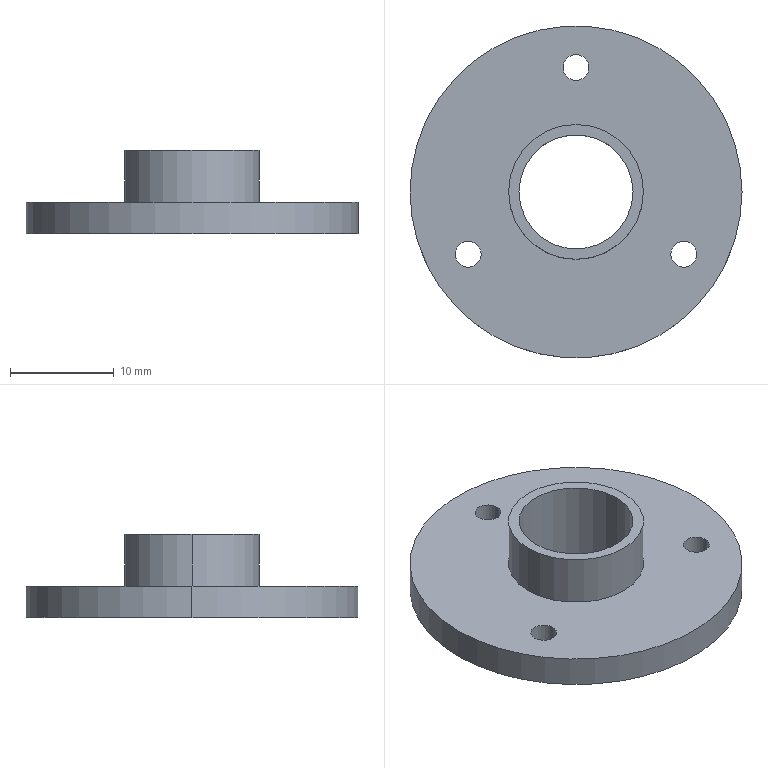Part | SolidWorks | features ICE 3, Extrusion 1, HoleWzd 1 | 1 solid | 15 faces | box 32 x 32 x 8 mm | volume 2272 mm3 | cylinder 12 | plane 3 | commonest cylinder face diameters 2.5 x6 11 x2 13 x2 32 x2
STEP:
#1=CARTESIAN_POINT('',(-1.25,12.,3.));
#2=VERTEX_POINT('',#1);
#3=CARTESIAN_POINT('',(1.25,12.,3.));
#4=VERTEX_POINT('',#3);
#5=CARTESIAN_POINT('',(0.,12.,3.));
#6=DIRECTION('',(0.,0.,1.));
#7=DIRECTION('',(1.,0.,0.));
#8=AXIS2_PLACEMENT_3D('',#5,#6,#7);
#9=CIRCLE('',#8,1.25);
#10=EDGE_CURVE('',#2,#4,#9,.T.);
#11=ORIENTED_EDGE('',*,*,#10,.T.);
#12=CARTESIAN_POINT('',(1.25,12.,0.));
#13=VERTEX_POINT('',#12);
#14=CARTESIAN_POINT('',(1.25,12.,0.));
#15=DIRECTION('',(0.,0.,-1.));
#16=VECTOR('',#15,1000.);
#17=LINE('',#14,#16);
#18=EDGE_CURVE('',#4,#13,#17,.T.);
#19=ORIENTED_EDGE('',*,*,#18,.T.);
#20=CARTESIAN_POINT('',(-1.25,12.,0.));
#21=VERTEX_POINT('',#20);
#22=CARTESIAN_POINT('',(0.,12.,0.));
#23=DIRECTION('',(0.,0.,-1.));
#24=DIRECTION('',(-1.,0.,0.));
#25=AXIS2_PLACEMENT_3D('',#22,#23,#24);
#26=CIRCLE('',#25,1.25);
#27=EDGE_CURVE('',#13,#21,#26,.T.);
#28=ORIENTED_EDGE('',*,*,#27,.T.);
#29=CARTESIAN_POINT('',(-1.25,12.,0.));
#30=DIRECTION('',(0.,0.,-1.));
#31=VECTOR('',#30,1000.);
#32=LINE('',#29,#31);
#33=EDGE_CURVE('',#2,#21,#32,.T.);
#34=ORIENTED_EDGE('',*,*,#33,.F.);
#35=EDGE_LOOP('',(#11,#19,#28,#34));
#36=FACE_OUTER_BOUND('',#35,.T.);
#37=CARTESIAN_POINT('',(0.,12.,0.));
#38=DIRECTION('',(0.,0.,-1.));
#39=DIRECTION('',(-1.,0.,0.));
#40=AXIS2_PLACEMENT_3D('',#37,#38,#39);
#41=CYLINDRICAL_SURFACE('',#40,1.25);
#42=ADVANCED_FACE('',(#36),#41,.F.);
#43=CARTESIAN_POINT('',(-11.642,-6.,3.));
#44=VERTEX_POINT('',#43);
#45=CARTESIAN_POINT('',(-9.142,-6.,3.));
#46=VERTEX_POINT('',#45);
#47=CARTESIAN_POINT('',(-10.392,-6.,3.));
#48=DIRECTION('',(0.,0.,1.));
#49=DIRECTION('',(1.,0.,0.));
#50=AXIS2_PLACEMENT_3D('',#47,#48,#49);
#51=CIRCLE('',#50,1.25);
#52=EDGE_CURVE('',#44,#46,#51,.T.);
#53=ORIENTED_EDGE('',*,*,#52,.T.);
#54=CARTESIAN_POINT('',(-9.142,-6.,0.));
#55=VERTEX_POINT('',#54);
#56=CARTESIAN_POINT('',(-9.142,-6.,0.));
#57=DIRECTION('',(0.,0.,-1.));
#58=VECTOR('',#57,1000.);
#59=LINE('',#56,#58);
#60=EDGE_CURVE('',#46,#55,#59,.T.);
#61=ORIENTED_EDGE('',*,*,#60,.T.);
#62=CARTESIAN_POINT('',(-11.642,-6.,0.));
#63=VERTEX_POINT('',#62);
#64=CARTESIAN_POINT('',(-10.392,-6.,0.));
#65=DIRECTION('',(0.,0.,-1.));
#66=DIRECTION('',(-1.,0.,0.));
#67=AXIS2_PLACEMENT_3D('',#64,#65,#66);
#68=CIRCLE('',#67,1.25);
#69=EDGE_CURVE('',#55,#63,#68,.T.);
#70=ORIENTED_EDGE('',*,*,#69,.T.);
#71=CARTESIAN_POINT('',(-11.642,-6.,0.));
#72=DIRECTION('',(0.,0.,-1.));
#73=VECTOR('',#72,1000.);
#74=LINE('',#71,#73);
#75=EDGE_CURVE('',#44,#63,#74,.T.);
#76=ORIENTED_EDGE('',*,*,#75,.F.);
#77=EDGE_LOOP('',(#53,#61,#70,#76));
#78=FACE_OUTER_BOUND('',#77,.T.);
#79=CARTESIAN_POINT('',(-10.392,-6.,0.));
#80=DIRECTION('',(0.,0.,-1.));
#81=DIRECTION('',(-1.,0.,0.));
#82=AXIS2_PLACEMENT_3D('',#79,#80,#81);
#83=CYLINDRICAL_SURFACE('',#82,1.25);
#84=ADVANCED_FACE('',(#78),#83,.F.);
#85=CARTESIAN_POINT('',(9.142,-6.,3.));
#86=VERTEX_POINT('',#85);
#87=CARTESIAN_POINT('',(11.642,-6.,3.));
#88=VERTEX_POINT('',#87);
#89=CARTESIAN_POINT('',(10.392,-6.,3.));
#90=DIRECTION('',(0.,0.,1.));
#91=DIRECTION('',(1.,0.,0.));
#92=AXIS2_PLACEMENT_3D('',#89,#90,#91);
#93=CIRCLE('',#92,1.25);
#94=EDGE_CURVE('',#86,#88,#93,.T.);
#95=ORIENTED_EDGE('',*,*,#94,.T.);
#96=CARTESIAN_POINT('',(11.642,-6.,0.));
#97=VERTEX_POINT('',#96);
#98=CARTESIAN_POINT('',(11.642,-6.,0.));
#99=DIRECTION('',(0.,0.,-1.));
#100=VECTOR('',#99,1000.);
#101=LINE('',#98,#100);
#102=EDGE_CURVE('',#88,#97,#101,.T.);
#103=ORIENTED_EDGE('',*,*,#102,.T.);
#104=CARTESIAN_POINT('',(9.142,-6.,0.));
#105=VERTEX_POINT('',#104);
#106=CARTESIAN_POINT('',(10.392,-6.,0.));
#107=DIRECTION('',(0.,0.,-1.));
#108=DIRECTION('',(-1.,0.,0.));
#109=AXIS2_PLACEMENT_3D('',#106,#107,#108);
#110=CIRCLE('',#109,1.25);
#111=EDGE_CURVE('',#97,#105,#110,.T.);
#112=ORIENTED_EDGE('',*,*,#111,.T.);
#113=CARTESIAN_POINT('',(9.142,-6.,0.));
#114=DIRECTION('',(0.,0.,-1.));
#115=VECTOR('',#114,1000.);
#116=LINE('',#113,#115);
#117=EDGE_CURVE('',#86,#105,#116,.T.);
#118=ORIENTED_EDGE('',*,*,#117,.F.);
#119=EDGE_LOOP('',(#95,#103,#112,#118));
#120=FACE_OUTER_BOUND('',#119,.T.);
#121=CARTESIAN_POINT('',(10.392,-6.,0.));
#122=DIRECTION('',(0.,0.,-1.));
#123=DIRECTION('',(-1.,0.,0.));
#124=AXIS2_PLACEMENT_3D('',#121,#122,#123);
#125=CYLINDRICAL_SURFACE('',#124,1.25);
#126=ADVANCED_FACE('',(#120),#125,.F.);
#127=CARTESIAN_POINT('',(-5.5,0.,8.));
#128=VERTEX_POINT('',#127);
#129=CARTESIAN_POINT('',(5.5,0.,8.));
#130=VERTEX_POINT('',#129);
#131=CARTESIAN_POINT('',(0.,0.,8.));
#132=DIRECTION('',(0.,0.,1.));
#133=DIRECTION('',(1.,0.,0.));
#134=AXIS2_PLACEMENT_3D('',#131,#132,#133);
#135=CIRCLE('',#134,5.5);
#136=EDGE_CURVE('',#128,#130,#135,.T.);
#137=ORIENTED_EDGE('',*,*,#136,.T.);
#138=CARTESIAN_POINT('',(5.5,0.,0.));
#139=VERTEX_POINT('',#138);
#140=CARTESIAN_POINT('',(5.5,0.,22.));
#141=DIRECTION('',(0.,0.,-1.));
#142=VECTOR('',#141,1000.);
#143=LINE('',#140,#142);
#144=EDGE_CURVE('',#130,#139,#143,.T.);
#145=ORIENTED_EDGE('',*,*,#144,.T.);
#146=CARTESIAN_POINT('',(-5.5,0.,0.));
#147=VERTEX_POINT('',#146);
#148=CARTESIAN_POINT('',(0.,0.,0.));
#149=DIRECTION('',(0.,0.,-1.));
#150=DIRECTION('',(-1.,0.,0.));
#151=AXIS2_PLACEMENT_3D('',#148,#149,#150);
#152=CIRCLE('',#151,5.5);
#153=EDGE_CURVE('',#139,#147,#152,.T.);
#154=ORIENTED_EDGE('',*,*,#153,.T.);
#155=CARTESIAN_POINT('',(-5.5,0.,22.));
#156=DIRECTION('',(0.,0.,-1.));
#157=VECTOR('',#156,1000.);
#158=LINE('',#155,#157);
#159=EDGE_CURVE('',#128,#147,#158,.T.);
#160=ORIENTED_EDGE('',*,*,#159,.F.);
#161=EDGE_LOOP('',(#137,#145,#154,#160));
#162=FACE_OUTER_BOUND('',#161,.T.);
#163=CARTESIAN_POINT('',(0.,0.,22.));
#164=DIRECTION('',(0.,0.,-1.));
#165=DIRECTION('',(-1.,0.,0.));
#166=AXIS2_PLACEMENT_3D('',#163,#164,#165);
#167=CYLINDRICAL_SURFACE('',#166,5.5);
#168=ADVANCED_FACE('',(#162),#167,.F.);
#169=CARTESIAN_POINT('',(6.5,0.,8.));
#170=VERTEX_POINT('',#169);
#171=CARTESIAN_POINT('',(-6.5,0.,8.));
#172=VERTEX_POINT('',#171);
#173=CARTESIAN_POINT('',(0.,0.,8.));
#174=DIRECTION('',(0.,0.,1.));
#175=DIRECTION('',(1.,0.,0.));
#176=AXIS2_PLACEMENT_3D('',#173,#174,#175);
#177=CIRCLE('',#176,6.5);
#178=EDGE_CURVE('',#170,#172,#177,.T.);
#179=ORIENTED_EDGE('',*,*,#178,.F.);
#180=CARTESIAN_POINT('',(6.5,0.,3.));
#181=VERTEX_POINT('',#180);
#182=CARTESIAN_POINT('',(6.5,0.,8.));
#183=DIRECTION('',(0.,0.,-1.));
#184=VECTOR('',#183,1000.);
#185=LINE('',#182,#184);
#186=EDGE_CURVE('',#170,#181,#185,.T.);
#187=ORIENTED_EDGE('',*,*,#186,.T.);
#188=CARTESIAN_POINT('',(-6.5,0.,3.));
#189=VERTEX_POINT('',#188);
#190=CARTESIAN_POINT('',(0.,0.,3.));
#191=DIRECTION('',(0.,0.,1.));
#192=DIRECTION('',(1.,0.,0.));
#193=AXIS2_PLACEMENT_3D('',#190,#191,#192);
#194=CIRCLE('',#193,6.5);
#195=EDGE_CURVE('',#181,#189,#194,.T.);
#196=ORIENTED_EDGE('',*,*,#195,.T.);
#197=CARTESIAN_POINT('',(-6.5,0.,8.));
#198=DIRECTION('',(0.,0.,-1.));
#199=VECTOR('',#198,1000.);
#200=LINE('',#197,#199);
#201=EDGE_CURVE('',#172,#189,#200,.T.);
#202=ORIENTED_EDGE('',*,*,#201,.F.);
#203=EDGE_LOOP('',(#179,#187,#196,#202));
#204=FACE_OUTER_BOUND('',#203,.T.);
#205=CARTESIAN_POINT('',(0.,0.,8.));
#206=DIRECTION('',(0.,0.,-1.));
#207=DIRECTION('',(-1.,0.,0.));
#208=AXIS2_PLACEMENT_3D('',#205,#206,#207);
#209=CYLINDRICAL_SURFACE('',#208,6.5);
#210=ADVANCED_FACE('',(#204),#209,.T.);
#211=CARTESIAN_POINT('',(16.,0.,3.));
#212=VERTEX_POINT('',#211);
#213=CARTESIAN_POINT('',(-16.,0.,3.));
#214=VERTEX_POINT('',#213);
#215=CARTESIAN_POINT('',(0.,0.,3.));
#216=DIRECTION('',(0.,0.,1.));
#217=DIRECTION('',(1.,0.,0.));
#218=AXIS2_PLACEMENT_3D('',#215,#216,#217);
#219=CIRCLE('',#218,16.);
#220=EDGE_CURVE('',#212,#214,#219,.T.);
#221=ORIENTED_EDGE('',*,*,#220,.F.);
#222=CARTESIAN_POINT('',(16.,0.,0.));
#223=VERTEX_POINT('',#222);
#224=CARTESIAN_POINT('',(16.,0.,3.));
#225=DIRECTION('',(0.,0.,-1.));
#226=VECTOR('',#225,1000.);
#227=LINE('',#224,#226);
#228=EDGE_CURVE('',#212,#223,#227,.T.);
#229=ORIENTED_EDGE('',*,*,#228,.T.);
#230=CARTESIAN_POINT('',(-16.,0.,0.));
#231=VERTEX_POINT('',#230);
#232=CARTESIAN_POINT('',(0.,0.,0.));
#233=DIRECTION('',(0.,0.,1.));
#234=DIRECTION('',(1.,0.,0.));
#235=AXIS2_PLACEMENT_3D('',#232,#233,#234);
#236=CIRCLE('',#235,16.);
#237=EDGE_CURVE('',#223,#231,#236,.T.);
#238=ORIENTED_EDGE('',*,*,#237,.T.);
#239=CARTESIAN_POINT('',(-16.,0.,3.));
#240=DIRECTION('',(0.,0.,-1.));
#241=VECTOR('',#240,1000.);
#242=LINE('',#239,#241);
#243=EDGE_CURVE('',#214,#231,#242,.T.);
#244=ORIENTED_EDGE('',*,*,#243,.F.);
#245=EDGE_LOOP('',(#221,#229,#238,#244));
#246=FACE_OUTER_BOUND('',#245,.T.);
#247=CARTESIAN_POINT('',(0.,0.,3.));
#248=DIRECTION('',(0.,0.,-1.));
#249=DIRECTION('',(-1.,0.,0.));
#250=AXIS2_PLACEMENT_3D('',#247,#248,#249);
#251=CYLINDRICAL_SURFACE('',#250,16.);
#252=ADVANCED_FACE('',(#246),#251,.T.);
#253=ORIENTED_EDGE('',*,*,#228,.F.);
#254=CARTESIAN_POINT('',(0.,0.,3.));
#255=DIRECTION('',(0.,0.,1.));
#256=DIRECTION('',(1.,0.,0.));
#257=AXIS2_PLACEMENT_3D('',#254,#255,#256);
#258=CIRCLE('',#257,16.);
#259=EDGE_CURVE('',#214,#212,#258,.T.);
#260=ORIENTED_EDGE('',*,*,#259,.F.);
#261=ORIENTED_EDGE('',*,*,#243,.T.);
#262=CARTESIAN_POINT('',(0.,0.,0.));
#263=DIRECTION('',(0.,0.,1.));
#264=DIRECTION('',(1.,0.,0.));
#265=AXIS2_PLACEMENT_3D('',#262,#263,#264);
#266=CIRCLE('',#265,16.);
#267=EDGE_CURVE('',#231,#223,#266,.T.);
#268=ORIENTED_EDGE('',*,*,#267,.T.);
#269=EDGE_LOOP('',(#253,#260,#261,#268));
#270=FACE_OUTER_BOUND('',#269,.T.);
#271=CARTESIAN_POINT('',(0.,0.,3.));
#272=DIRECTION('',(0.,0.,-1.));
#273=DIRECTION('',(-1.,0.,0.));
#274=AXIS2_PLACEMENT_3D('',#271,#272,#273);
#275=CYLINDRICAL_SURFACE('',#274,16.);
#276=ADVANCED_FACE('',(#270),#275,.T.);
#277=ORIENTED_EDGE('',*,*,#10,.F.);
#278=CARTESIAN_POINT('',(0.,12.,3.));
#279=DIRECTION('',(0.,0.,1.));
#280=DIRECTION('',(1.,0.,0.));
#281=AXIS2_PLACEMENT_3D('',#278,#279,#280);
#282=CIRCLE('',#281,1.25);
#283=EDGE_CURVE('',#4,#2,#282,.T.);
#284=ORIENTED_EDGE('',*,*,#283,.F.);
#285=EDGE_LOOP('',(#277,#284));
#286=FACE_BOUND('',#285,.T.);
#287=ORIENTED_EDGE('',*,*,#52,.F.);
#288=CARTESIAN_POINT('',(-10.392,-6.,3.));
#289=DIRECTION('',(0.,0.,1.));
#290=DIRECTION('',(1.,0.,0.));
#291=AXIS2_PLACEMENT_3D('',#288,#289,#290);
#292=CIRCLE('',#291,1.25);
#293=EDGE_CURVE('',#46,#44,#292,.T.);
#294=ORIENTED_EDGE('',*,*,#293,.F.);
#295=EDGE_LOOP('',(#287,#294));
#296=FACE_BOUND('',#295,.T.);
#297=ORIENTED_EDGE('',*,*,#94,.F.);
#298=CARTESIAN_POINT('',(10.392,-6.,3.));
#299=DIRECTION('',(0.,0.,1.));
#300=DIRECTION('',(1.,0.,0.));
#301=AXIS2_PLACEMENT_3D('',#298,#299,#300);
#302=CIRCLE('',#301,1.25);
#303=EDGE_CURVE('',#88,#86,#302,.T.);
#304=ORIENTED_EDGE('',*,*,#303,.F.);
#305=EDGE_LOOP('',(#297,#304));
#306=FACE_BOUND('',#305,.T.);
#307=CARTESIAN_POINT('',(0.,0.,3.));
#308=DIRECTION('',(0.,0.,1.));
#309=DIRECTION('',(1.,0.,0.));
#310=AXIS2_PLACEMENT_3D('',#307,#308,#309);
#311=CIRCLE('',#310,6.5);
#312=EDGE_CURVE('',#189,#181,#311,.T.);
#313=ORIENTED_EDGE('',*,*,#312,.F.);
#314=ORIENTED_EDGE('',*,*,#195,.F.);
#315=EDGE_LOOP('',(#313,#314));
#316=FACE_BOUND('',#315,.T.);
#317=ORIENTED_EDGE('',*,*,#259,.T.);
#318=ORIENTED_EDGE('',*,*,#220,.T.);
#319=EDGE_LOOP('',(#317,#318));
#320=FACE_OUTER_BOUND('',#319,.T.);
#321=CARTESIAN_POINT('',(0.,0.,3.));
#322=DIRECTION('',(0.,0.,1.));
#323=DIRECTION('',(1.,0.,0.));
#324=AXIS2_PLACEMENT_3D('',#321,#322,#323);
#325=PLANE('',#324);
#326=ADVANCED_FACE('',(#286,#296,#306,#316,#320),#325,.T.);
#327=CARTESIAN_POINT('',(0.,12.,0.));
#328=DIRECTION('',(0.,0.,-1.));
#329=DIRECTION('',(-1.,0.,0.));
#330=AXIS2_PLACEMENT_3D('',#327,#328,#329);
#331=CIRCLE('',#330,1.25);
#332=EDGE_CURVE('',#21,#13,#331,.T.);
#333=ORIENTED_EDGE('',*,*,#332,.F.);
#334=ORIENTED_EDGE('',*,*,#27,.F.);
#335=EDGE_LOOP('',(#333,#334));
#336=FACE_BOUND('',#335,.T.);
#337=CARTESIAN_POINT('',(-10.392,-6.,0.));
#338=DIRECTION('',(0.,0.,-1.));
#339=DIRECTION('',(-1.,0.,0.));
#340=AXIS2_PLACEMENT_3D('',#337,#338,#339);
#341=CIRCLE('',#340,1.25);
#342=EDGE_CURVE('',#63,#55,#341,.T.);
#343=ORIENTED_EDGE('',*,*,#342,.F.);
#344=ORIENTED_EDGE('',*,*,#69,.F.);
#345=EDGE_LOOP('',(#343,#344));
#346=FACE_BOUND('',#345,.T.);
#347=CARTESIAN_POINT('',(10.392,-6.,0.));
#348=DIRECTION('',(0.,0.,-1.));
#349=DIRECTION('',(-1.,0.,0.));
#350=AXIS2_PLACEMENT_3D('',#347,#348,#349);
#351=CIRCLE('',#350,1.25);
#352=EDGE_CURVE('',#105,#97,#351,.T.);
#353=ORIENTED_EDGE('',*,*,#352,.F.);
#354=ORIENTED_EDGE('',*,*,#111,.F.);
#355=EDGE_LOOP('',(#353,#354));
#356=FACE_BOUND('',#355,.T.);
#357=CARTESIAN_POINT('',(0.,0.,0.));
#358=DIRECTION('',(0.,0.,-1.));
#359=DIRECTION('',(-1.,0.,0.));
#360=AXIS2_PLACEMENT_3D('',#357,#358,#359);
#361=CIRCLE('',#360,5.5);
#362=EDGE_CURVE('',#147,#139,#361,.T.);
#363=ORIENTED_EDGE('',*,*,#362,.F.);
#364=ORIENTED_EDGE('',*,*,#153,.F.);
#365=EDGE_LOOP('',(#363,#364));
#366=FACE_BOUND('',#365,.T.);
#367=ORIENTED_EDGE('',*,*,#267,.F.);
#368=ORIENTED_EDGE('',*,*,#237,.F.);
#369=EDGE_LOOP('',(#367,#368));
#370=FACE_OUTER_BOUND('',#369,.T.);
#371=CARTESIAN_POINT('',(0.,0.,0.));
#372=DIRECTION('',(0.,0.,1.));
#373=DIRECTION('',(1.,0.,0.));
#374=AXIS2_PLACEMENT_3D('',#371,#372,#373);
#375=PLANE('',#374);
#376=ADVANCED_FACE('',(#336,#346,#356,#366,#370),#375,.F.);
#377=ORIENTED_EDGE('',*,*,#186,.F.);
#378=CARTESIAN_POINT('',(0.,0.,8.));
#379=DIRECTION('',(0.,0.,1.));
#380=DIRECTION('',(1.,0.,0.));
#381=AXIS2_PLACEMENT_3D('',#378,#379,#380);
#382=CIRCLE('',#381,6.5);
#383=EDGE_CURVE('',#172,#170,#382,.T.);
#384=ORIENTED_EDGE('',*,*,#383,.F.);
#385=ORIENTED_EDGE('',*,*,#201,.T.);
#386=ORIENTED_EDGE('',*,*,#312,.T.);
#387=EDGE_LOOP('',(#377,#384,#385,#386));
#388=FACE_OUTER_BOUND('',#387,.T.);
#389=CARTESIAN_POINT('',(0.,0.,8.));
#390=DIRECTION('',(0.,0.,-1.));
#391=DIRECTION('',(-1.,0.,0.));
#392=AXIS2_PLACEMENT_3D('',#389,#390,#391);
#393=CYLINDRICAL_SURFACE('',#392,6.5);
#394=ADVANCED_FACE('',(#388),#393,.T.);
#395=ORIENTED_EDGE('',*,*,#136,.F.);
#396=CARTESIAN_POINT('',(0.,0.,8.));
#397=DIRECTION('',(0.,0.,1.));
#398=DIRECTION('',(1.,0.,0.));
#399=AXIS2_PLACEMENT_3D('',#396,#397,#398);
#400=CIRCLE('',#399,5.5);
#401=EDGE_CURVE('',#130,#128,#400,.T.);
#402=ORIENTED_EDGE('',*,*,#401,.F.);
#403=EDGE_LOOP('',(#395,#402));
#404=FACE_BOUND('',#403,.T.);
#405=ORIENTED_EDGE('',*,*,#383,.T.);
#406=ORIENTED_EDGE('',*,*,#178,.T.);
#407=EDGE_LOOP('',(#405,#406));
#408=FACE_OUTER_BOUND('',#407,.T.);
#409=CARTESIAN_POINT('',(0.,0.,8.));
#410=DIRECTION('',(0.,0.,1.));
#411=DIRECTION('',(1.,0.,0.));
#412=AXIS2_PLACEMENT_3D('',#409,#410,#411);
#413=PLANE('',#412);
#414=ADVANCED_FACE('',(#404,#408),#413,.T.);
#415=ORIENTED_EDGE('',*,*,#144,.F.);
#416=ORIENTED_EDGE('',*,*,#401,.T.);
#417=ORIENTED_EDGE('',*,*,#159,.T.);
#418=ORIENTED_EDGE('',*,*,#362,.T.);
#419=EDGE_LOOP('',(#415,#416,#417,#418));
#420=FACE_OUTER_BOUND('',#419,.T.);
#421=CARTESIAN_POINT('',(0.,0.,22.));
#422=DIRECTION('',(0.,0.,-1.));
#423=DIRECTION('',(-1.,0.,0.));
#424=AXIS2_PLACEMENT_3D('',#421,#422,#423);
#425=CYLINDRICAL_SURFACE('',#424,5.5);
#426=ADVANCED_FACE('',(#420),#425,.F.);
#427=ORIENTED_EDGE('',*,*,#102,.F.);
#428=ORIENTED_EDGE('',*,*,#303,.T.);
#429=ORIENTED_EDGE('',*,*,#117,.T.);
#430=ORIENTED_EDGE('',*,*,#352,.T.);
#431=EDGE_LOOP('',(#427,#428,#429,#430));
#432=FACE_OUTER_BOUND('',#431,.T.);
#433=CARTESIAN_POINT('',(10.392,-6.,0.));
#434=DIRECTION('',(0.,0.,-1.));
#435=DIRECTION('',(-1.,0.,0.));
#436=AXIS2_PLACEMENT_3D('',#433,#434,#435);
#437=CYLINDRICAL_SURFACE('',#436,1.25);
#438=ADVANCED_FACE('',(#432),#437,.F.);
#439=ORIENTED_EDGE('',*,*,#60,.F.);
#440=ORIENTED_EDGE('',*,*,#293,.T.);
#441=ORIENTED_EDGE('',*,*,#75,.T.);
#442=ORIENTED_EDGE('',*,*,#342,.T.);
#443=EDGE_LOOP('',(#439,#440,#441,#442));
#444=FACE_OUTER_BOUND('',#443,.T.);
#445=CARTESIAN_POINT('',(-10.392,-6.,0.));
#446=DIRECTION('',(0.,0.,-1.));
#447=DIRECTION('',(-1.,0.,0.));
#448=AXIS2_PLACEMENT_3D('',#445,#446,#447);
#449=CYLINDRICAL_SURFACE('',#448,1.25);
#450=ADVANCED_FACE('',(#444),#449,.F.);
#451=ORIENTED_EDGE('',*,*,#18,.F.);
#452=ORIENTED_EDGE('',*,*,#283,.T.);
#453=ORIENTED_EDGE('',*,*,#33,.T.);
#454=ORIENTED_EDGE('',*,*,#332,.T.);
#455=EDGE_LOOP('',(#451,#452,#453,#454));
#456=FACE_OUTER_BOUND('',#455,.T.);
#457=CARTESIAN_POINT('',(0.,12.,0.));
#458=DIRECTION('',(0.,0.,-1.));
#459=DIRECTION('',(-1.,0.,0.));
#460=AXIS2_PLACEMENT_3D('',#457,#458,#459);
#461=CYLINDRICAL_SURFACE('',#460,1.25);
#462=ADVANCED_FACE('',(#456),#461,.F.);
#463=CLOSED_SHELL('',(#42,#84,#126,#168,#210,#252,#276,#326,#376,#394,#414,#426,#438,#450,#462));
#464=MANIFOLD_SOLID_BREP('',#463);
#465=CARTESIAN_POINT('',(0.,0.,0.));
#466=DIRECTION('',(0.,0.,1.));
#467=DIRECTION('',(1.,0.,0.));
#468=AXIS2_PLACEMENT_3D('',#465,#466,#467);
#469=(LENGTH_UNIT()NAMED_UNIT(*)SI_UNIT(.MILLI.,.METRE.));
#470=UNCERTAINTY_MEASURE_WITH_UNIT(LENGTH_MEASURE(0.00001),#469,'','');
#471=(NAMED_UNIT(*)PLANE_ANGLE_UNIT()SI_UNIT($,.RADIAN.));
#472=(NAMED_UNIT(*)SI_UNIT($,.STERADIAN.)SOLID_ANGLE_UNIT());
#473=(GEOMETRIC_REPRESENTATION_CONTEXT(3)GLOBAL_UNCERTAINTY_ASSIGNED_CONTEXT((#470))GLOBAL_UNIT_ASSIGNED_CONTEXT((#469,#471,#472))REPRESENTATION_CONTEXT('',''));
#474=ADVANCED_BREP_SHAPE_REPRESENTATION('',(#464,#468),#473);